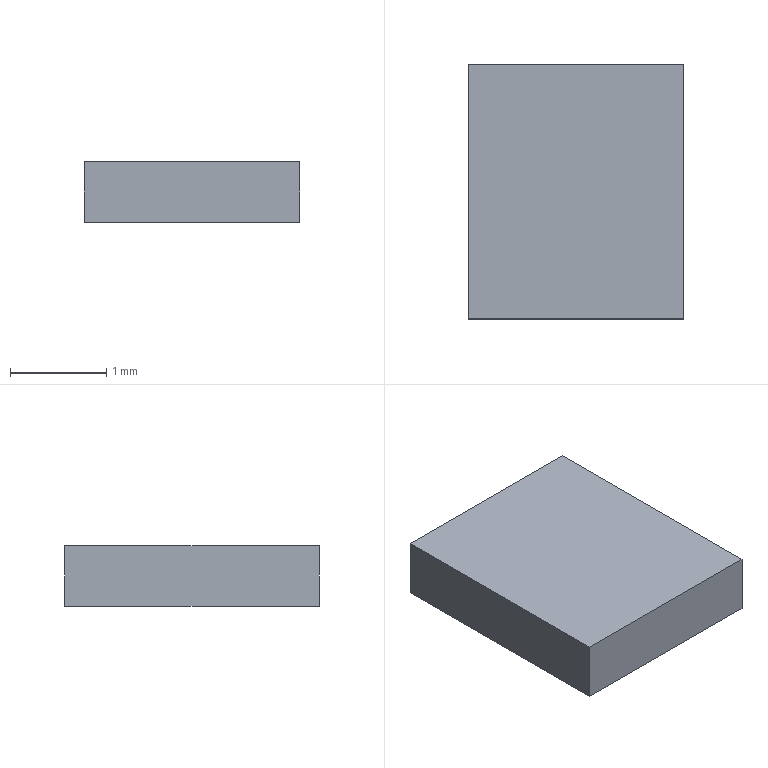Part | Creo | 1 solid | 6 faces | box 2.236 x 2.636 x 0.6251 mm | volume 3.684 mm3 | plane 6
STEP:
#1=CARTESIAN_POINT('',(0.,0.,0.));
#2=DIRECTION('',(0.,0.,1.));
#3=DIRECTION('',(1.,0.,0.));
#4=AXIS2_PLACEMENT_3D('',#1,#2,#3);
#5=CARTESIAN_POINT('',(-1.236,-1.2,0.));
#6=VERTEX_POINT('',#5);
#7=CARTESIAN_POINT('',(1.,-1.2,0.));
#8=VERTEX_POINT('',#7);
#9=CARTESIAN_POINT('',(-1.236,-1.2,0.));
#10=DIRECTION('',(1.,0.,0.));
#11=VECTOR('',#10,2.236);
#12=LINE('',#9,#11);
#13=EDGE_CURVE('',#6,#8,#12,.T.);
#14=ORIENTED_EDGE('',*,*,#13,.T.);
#15=CARTESIAN_POINT('',(1.,1.436,0.));
#16=VERTEX_POINT('',#15);
#17=CARTESIAN_POINT('',(1.,-1.2,0.));
#18=DIRECTION('',(0.,1.,0.));
#19=VECTOR('',#18,2.636);
#20=LINE('',#17,#19);
#21=EDGE_CURVE('',#8,#16,#20,.T.);
#22=ORIENTED_EDGE('',*,*,#21,.T.);
#23=CARTESIAN_POINT('',(-1.236,1.436,0.));
#24=VERTEX_POINT('',#23);
#25=CARTESIAN_POINT('',(1.,1.436,0.));
#26=DIRECTION('',(-1.,0.,0.));
#27=VECTOR('',#26,2.236);
#28=LINE('',#25,#27);
#29=EDGE_CURVE('',#16,#24,#28,.T.);
#30=ORIENTED_EDGE('',*,*,#29,.T.);
#31=CARTESIAN_POINT('',(-1.236,1.436,0.));
#32=DIRECTION('',(0.,-1.,0.));
#33=VECTOR('',#32,2.636);
#34=LINE('',#31,#33);
#35=EDGE_CURVE('',#24,#6,#34,.T.);
#36=ORIENTED_EDGE('',*,*,#35,.T.);
#37=EDGE_LOOP('',(#14,#22,#30,#36));
#38=FACE_OUTER_BOUND('',#37,.F.);
#39=CARTESIAN_POINT('',(0.,0.,0.));
#40=DIRECTION('',(0.,0.,1.));
#41=DIRECTION('',(1.,0.,0.));
#42=AXIS2_PLACEMENT_3D('',#39,#40,#41);
#43=PLANE('',#42);
#44=ADVANCED_FACE('',(#38),#43,.F.);
#45=ORIENTED_EDGE('',*,*,#13,.F.);
#46=CARTESIAN_POINT('',(-1.236,-1.2,0.6251));
#47=VERTEX_POINT('',#46);
#48=CARTESIAN_POINT('',(-1.236,-1.2,0.));
#49=DIRECTION('',(0.,0.,1.));
#50=VECTOR('',#49,0.6251);
#51=LINE('',#48,#50);
#52=EDGE_CURVE('',#6,#47,#51,.T.);
#53=ORIENTED_EDGE('',*,*,#52,.T.);
#54=CARTESIAN_POINT('',(1.,-1.2,0.6251));
#55=VERTEX_POINT('',#54);
#56=CARTESIAN_POINT('',(-1.236,-1.2,0.6251));
#57=DIRECTION('',(1.,0.,0.));
#58=VECTOR('',#57,2.236);
#59=LINE('',#56,#58);
#60=EDGE_CURVE('',#47,#55,#59,.T.);
#61=ORIENTED_EDGE('',*,*,#60,.T.);
#62=CARTESIAN_POINT('',(1.,-1.2,0.));
#63=DIRECTION('',(0.,0.,1.));
#64=VECTOR('',#63,0.6251);
#65=LINE('',#62,#64);
#66=EDGE_CURVE('',#8,#55,#65,.T.);
#67=ORIENTED_EDGE('',*,*,#66,.F.);
#68=EDGE_LOOP('',(#45,#53,#61,#67));
#69=FACE_OUTER_BOUND('',#68,.F.);
#70=CARTESIAN_POINT('',(-1.236,-1.2,0.));
#71=DIRECTION('',(0.,-1.,0.));
#72=DIRECTION('',(1.,0.,0.));
#73=AXIS2_PLACEMENT_3D('',#70,#71,#72);
#74=PLANE('',#73);
#75=ADVANCED_FACE('',(#69),#74,.T.);
#76=ORIENTED_EDGE('',*,*,#35,.F.);
#77=CARTESIAN_POINT('',(-1.236,1.436,0.6251));
#78=VERTEX_POINT('',#77);
#79=CARTESIAN_POINT('',(-1.236,1.436,0.));
#80=DIRECTION('',(0.,0.,1.));
#81=VECTOR('',#80,0.6251);
#82=LINE('',#79,#81);
#83=EDGE_CURVE('',#24,#78,#82,.T.);
#84=ORIENTED_EDGE('',*,*,#83,.T.);
#85=CARTESIAN_POINT('',(-1.236,1.436,0.6251));
#86=DIRECTION('',(0.,-1.,0.));
#87=VECTOR('',#86,2.636);
#88=LINE('',#85,#87);
#89=EDGE_CURVE('',#78,#47,#88,.T.);
#90=ORIENTED_EDGE('',*,*,#89,.T.);
#91=ORIENTED_EDGE('',*,*,#52,.F.);
#92=EDGE_LOOP('',(#76,#84,#90,#91));
#93=FACE_OUTER_BOUND('',#92,.F.);
#94=CARTESIAN_POINT('',(-1.236,1.436,0.));
#95=DIRECTION('',(-1.,0.,0.));
#96=DIRECTION('',(0.,-1.,0.));
#97=AXIS2_PLACEMENT_3D('',#94,#95,#96);
#98=PLANE('',#97);
#99=ADVANCED_FACE('',(#93),#98,.T.);
#100=ORIENTED_EDGE('',*,*,#29,.F.);
#101=CARTESIAN_POINT('',(1.,1.436,0.6251));
#102=VERTEX_POINT('',#101);
#103=CARTESIAN_POINT('',(1.,1.436,0.));
#104=DIRECTION('',(0.,0.,1.));
#105=VECTOR('',#104,0.6251);
#106=LINE('',#103,#105);
#107=EDGE_CURVE('',#16,#102,#106,.T.);
#108=ORIENTED_EDGE('',*,*,#107,.T.);
#109=CARTESIAN_POINT('',(1.,1.436,0.6251));
#110=DIRECTION('',(-1.,0.,0.));
#111=VECTOR('',#110,2.236);
#112=LINE('',#109,#111);
#113=EDGE_CURVE('',#102,#78,#112,.T.);
#114=ORIENTED_EDGE('',*,*,#113,.T.);
#115=ORIENTED_EDGE('',*,*,#83,.F.);
#116=EDGE_LOOP('',(#100,#108,#114,#115));
#117=FACE_OUTER_BOUND('',#116,.F.);
#118=CARTESIAN_POINT('',(1.,1.436,0.));
#119=DIRECTION('',(0.,1.,0.));
#120=DIRECTION('',(-1.,0.,0.));
#121=AXIS2_PLACEMENT_3D('',#118,#119,#120);
#122=PLANE('',#121);
#123=ADVANCED_FACE('',(#117),#122,.T.);
#124=ORIENTED_EDGE('',*,*,#21,.F.);
#125=ORIENTED_EDGE('',*,*,#66,.T.);
#126=CARTESIAN_POINT('',(1.,-1.2,0.6251));
#127=DIRECTION('',(0.,1.,0.));
#128=VECTOR('',#127,2.636);
#129=LINE('',#126,#128);
#130=EDGE_CURVE('',#55,#102,#129,.T.);
#131=ORIENTED_EDGE('',*,*,#130,.T.);
#132=ORIENTED_EDGE('',*,*,#107,.F.);
#133=EDGE_LOOP('',(#124,#125,#131,#132));
#134=FACE_OUTER_BOUND('',#133,.F.);
#135=CARTESIAN_POINT('',(1.,-1.2,0.));
#136=DIRECTION('',(1.,0.,0.));
#137=DIRECTION('',(0.,1.,0.));
#138=AXIS2_PLACEMENT_3D('',#135,#136,#137);
#139=PLANE('',#138);
#140=ADVANCED_FACE('',(#134),#139,.T.);
#141=ORIENTED_EDGE('',*,*,#60,.F.);
#142=ORIENTED_EDGE('',*,*,#89,.F.);
#143=ORIENTED_EDGE('',*,*,#113,.F.);
#144=ORIENTED_EDGE('',*,*,#130,.F.);
#145=EDGE_LOOP('',(#141,#142,#143,#144));
#146=FACE_OUTER_BOUND('',#145,.F.);
#147=CARTESIAN_POINT('',(0.,0.,0.6251));
#148=DIRECTION('',(0.,0.,1.));
#149=DIRECTION('',(1.,0.,0.));
#150=AXIS2_PLACEMENT_3D('',#147,#148,#149);
#151=PLANE('',#150);
#152=ADVANCED_FACE('',(#146),#151,.T.);
#153=CLOSED_SHELL('',(#44,#75,#99,#123,#140,#152));
#154=MANIFOLD_SOLID_BREP('',#153);
#155=(LENGTH_UNIT()NAMED_UNIT(*)SI_UNIT(.MILLI.,.METRE.));
#156=UNCERTAINTY_MEASURE_WITH_UNIT(LENGTH_MEASURE(0.0003513),#155,'','');
#157=(NAMED_UNIT(*)PLANE_ANGLE_UNIT()SI_UNIT($,.RADIAN.));
#158=PLANE_ANGLE_MEASURE_WITH_UNIT(PLANE_ANGLE_MEASURE(0.01745),#157);
#159=(CONVERSION_BASED_UNIT('DEGREE',#158)NAMED_UNIT(*)PLANE_ANGLE_UNIT());
#160=(NAMED_UNIT(*)SI_UNIT($,.STERADIAN.)SOLID_ANGLE_UNIT());
#161=(GEOMETRIC_REPRESENTATION_CONTEXT(3)GLOBAL_UNCERTAINTY_ASSIGNED_CONTEXT((#156))GLOBAL_UNIT_ASSIGNED_CONTEXT((#155,#159,#160))REPRESENTATION_CONTEXT('',''));
#162=ADVANCED_BREP_SHAPE_REPRESENTATION('',(#4,#154),#161);